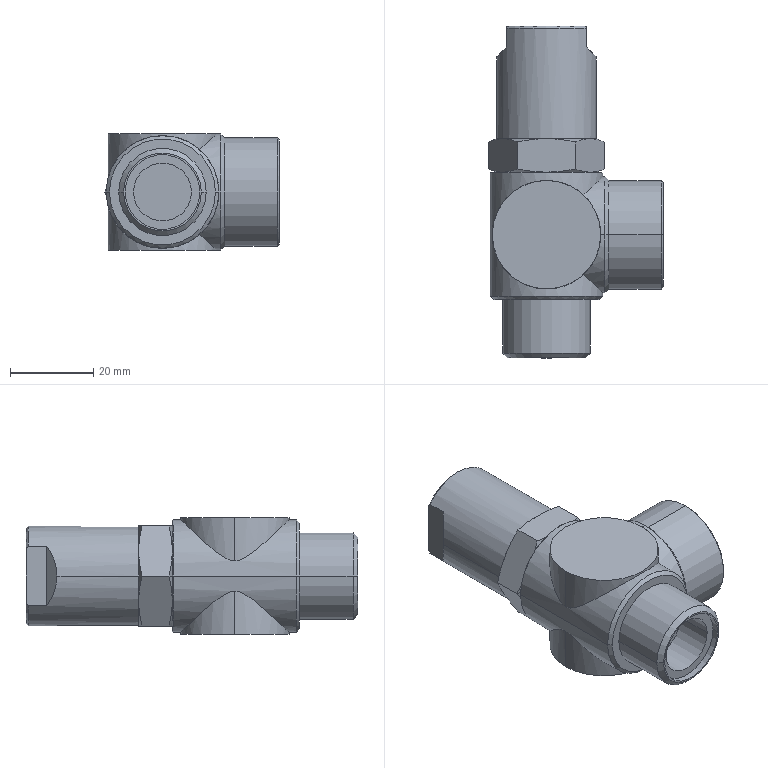Part | STEP file | PCV15 | 1 solid | 74 faces | box 41.856 x 79.5 x 28 mm | volume 41783 mm3 | cone 30 | cylinder 22 | plane 22 | commonest cylinder face diameters 26 x6 11.445 x2 13.895 x2 17.895 x2 18.631 x2 20.955 x2